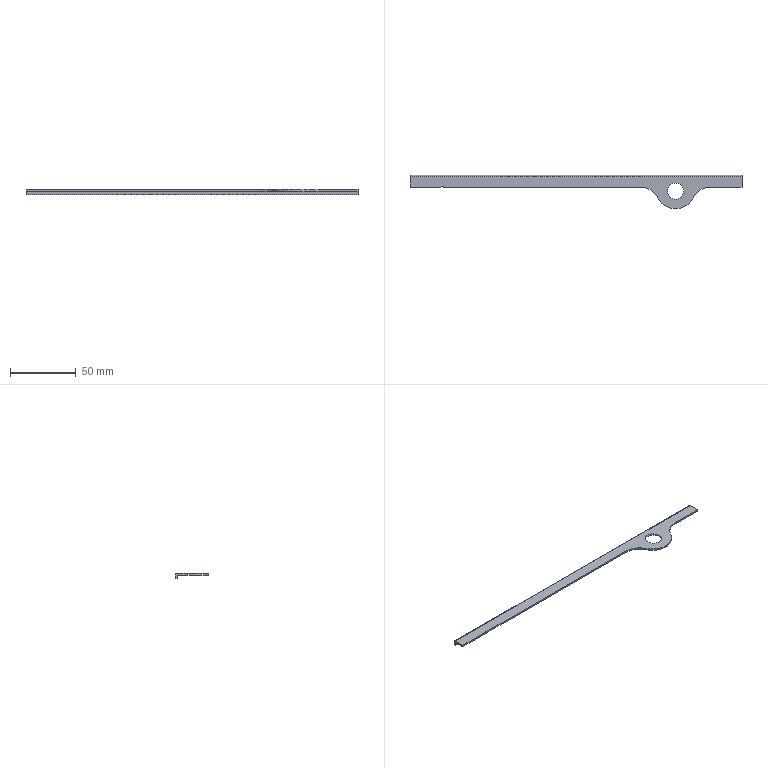Part | STEP file | gslz 2016.10.28-13_id1034_x_t | 1 solid | 17 faces | box 253.449 x 25.5 x 4 mm | volume 4072 mm3 | plane 10 | cylinder 7 | commonest cylinder face diameters 30 x3 4 x2 2 x1 12.3 x1
STEP:
#1=CARTESIAN_POINT('',(0.,0.,0.));
#2=DIRECTION('',(0.,0.,1.));
#3=DIRECTION('',(1.,0.,0.));
#4=AXIS2_PLACEMENT_3D('',#1,#2,#3);
#5=CARTESIAN_POINT('',(1262.778,254.,1.25));
#6=VERTEX_POINT('',#5);
#7=CARTESIAN_POINT('',(1256.628,254.,1.25));
#8=DIRECTION('',(0.,0.,1.));
#9=DIRECTION('',(1.,0.,0.));
#10=AXIS2_PLACEMENT_3D('',#7,#8,#9);
#11=CIRCLE('',#10,6.15);
#12=CARTESIAN_POINT('',(1256.628,254.,2.5));
#13=DIRECTION('',(0.,0.,-1.));
#14=DIRECTION('',(-1.,0.,0.));
#15=AXIS2_PLACEMENT_3D('',#12,#13,#14);
#16=CYLINDRICAL_SURFACE('',#15,6.15);
#17=CARTESIAN_POINT('',(9.425,1.25));
#18=DIRECTION('',(-1.,0.));
#19=VECTOR('',#18,1.);
#20=LINE('',#17,#19);
#21=(GEOMETRIC_REPRESENTATION_CONTEXT(2)PARAMETRIC_REPRESENTATION_CONTEXT()REPRESENTATION_CONTEXT('',''));
#22=DEFINITIONAL_REPRESENTATION('',(#20),#21);
#23=PCURVE('',#16,#22);
#24=CARTESIAN_POINT('',(3468.591,331.067,1.25));
#25=DIRECTION('',(0.,0.,1.));
#26=DIRECTION('',(1.,0.,0.));
#27=AXIS2_PLACEMENT_3D('',#24,#25,#26);
#28=PLANE('',#27);
#29=CARTESIAN_POINT('',(-2211.964,-77.067));
#30=DIRECTION('',(1.,0.));
#31=AXIS2_PLACEMENT_2D('',#29,#30);
#32=CIRCLE('',#31,6.15);
#33=(GEOMETRIC_REPRESENTATION_CONTEXT(2)PARAMETRIC_REPRESENTATION_CONTEXT()REPRESENTATION_CONTEXT('',''));
#34=DEFINITIONAL_REPRESENTATION('',(#32),#33);
#35=PCURVE('',#28,#34);
#36=SURFACE_CURVE('',#11,(#23,#35),.PCURVE_S1.);
#37=EDGE_CURVE('',#6,#6,#36,.T.);
#38=ORIENTED_EDGE('',*,*,#37,.F.);
#39=CARTESIAN_POINT('',(1262.778,254.,0.));
#40=VERTEX_POINT('',#39);
#41=CARTESIAN_POINT('',(1262.778,254.,1.25));
#42=CARTESIAN_POINT('',(1262.778,254.,0.));
#43=B_SPLINE_CURVE_WITH_KNOTS('',1,(#41,#42),.UNSPECIFIED.,.F.,.F.,(2,2),(1.25,2.5),.PIECEWISE_BEZIER_KNOTS.);
#44=CARTESIAN_POINT('',(9.425,0.));
#45=DIRECTION('',(0.,1.));
#46=VECTOR('',#45,1.);
#47=LINE('',#44,#46);
#48=(GEOMETRIC_REPRESENTATION_CONTEXT(2)PARAMETRIC_REPRESENTATION_CONTEXT()REPRESENTATION_CONTEXT('',''));
#49=DEFINITIONAL_REPRESENTATION('',(#47),#48);
#50=PCURVE('',#16,#49);
#51=CARTESIAN_POINT('',(3.142,0.));
#52=DIRECTION('',(0.,1.));
#53=VECTOR('',#52,1.);
#54=LINE('',#51,#53);
#55=(GEOMETRIC_REPRESENTATION_CONTEXT(2)PARAMETRIC_REPRESENTATION_CONTEXT()REPRESENTATION_CONTEXT('',''));
#56=DEFINITIONAL_REPRESENTATION('',(#54),#55);
#57=PCURVE('',#16,#56);
#58=SEAM_CURVE('',#43,(#50,#57),.PCURVE_S1.);
#59=EDGE_CURVE('',#6,#40,#58,.T.);
#60=ORIENTED_EDGE('',*,*,#59,.T.);
#61=CARTESIAN_POINT('',(1256.628,254.,0.));
#62=DIRECTION('',(0.,0.,-1.));
#63=DIRECTION('',(1.,0.,0.));
#64=AXIS2_PLACEMENT_3D('',#61,#62,#63);
#65=CIRCLE('',#64,6.15);
#66=CARTESIAN_POINT('',(3.142,2.5));
#67=DIRECTION('',(1.,0.));
#68=VECTOR('',#67,1.);
#69=LINE('',#66,#68);
#70=(GEOMETRIC_REPRESENTATION_CONTEXT(2)PARAMETRIC_REPRESENTATION_CONTEXT()REPRESENTATION_CONTEXT('',''));
#71=DEFINITIONAL_REPRESENTATION('',(#69),#70);
#72=PCURVE('',#16,#71);
#73=CARTESIAN_POINT('',(3468.591,331.067,0.));
#74=DIRECTION('',(0.,0.,1.));
#75=DIRECTION('',(1.,0.,0.));
#76=AXIS2_PLACEMENT_3D('',#73,#74,#75);
#77=PLANE('',#76);
#78=CARTESIAN_POINT('',(-2205.814,-77.067));
#79=CARTESIAN_POINT('',(-2205.814,-87.719));
#80=CARTESIAN_POINT('',(-2215.039,-82.393));
#81=CARTESIAN_POINT('',(-2224.264,-77.067));
#82=CARTESIAN_POINT('',(-2215.039,-71.741));
#83=CARTESIAN_POINT('',(-2205.814,-66.415));
#84=CARTESIAN_POINT('',(-2205.814,-77.067));
#85=(BOUNDED_CURVE()B_SPLINE_CURVE(2,(#78,#79,#80,#81,#82,#83,#84),.UNSPECIFIED.,.T.,.F.)B_SPLINE_CURVE_WITH_KNOTS((1,2,2,2,2,1),(-2.094,0.,2.094,4.189,6.283,8.378),.UNSPECIFIED.)CURVE()GEOMETRIC_REPRESENTATION_ITEM()RATIONAL_B_SPLINE_CURVE((1.,0.5,1.,0.5,1.,0.5,1.))REPRESENTATION_ITEM(''));
#86=(GEOMETRIC_REPRESENTATION_CONTEXT(2)PARAMETRIC_REPRESENTATION_CONTEXT()REPRESENTATION_CONTEXT('',''));
#87=DEFINITIONAL_REPRESENTATION('',(#85),#86);
#88=PCURVE('',#77,#87);
#89=SURFACE_CURVE('',#65,(#72,#88),.PCURVE_S1.);
#90=EDGE_CURVE('',#40,#40,#89,.T.);
#91=ORIENTED_EDGE('',*,*,#90,.F.);
#92=ORIENTED_EDGE('',*,*,#59,.F.);
#93=EDGE_LOOP('',(#38,#60,#91,#92));
#94=FACE_BOUND('',#93,.F.);
#95=ADVANCED_FACE('',(#94),#16,.F.);
#96=CARTESIAN_POINT('',(1077.412,257.,1.25));
#97=VERTEX_POINT('',#96);
#98=CARTESIAN_POINT('',(1053.925,257.,1.25));
#99=VERTEX_POINT('',#98);
#100=CARTESIAN_POINT('',(3468.591,257.,1.25));
#101=DIRECTION('',(-1.,0.,0.));
#102=VECTOR('',#101,1.);
#103=LINE('',#100,#102);
#104=CARTESIAN_POINT('',(1000.415,257.,2.5));
#105=DIRECTION('',(0.,1.,0.));
#106=DIRECTION('',(0.,0.,1.));
#107=AXIS2_PLACEMENT_3D('',#104,#105,#106);
#108=PLANE('',#107);
#109=CARTESIAN_POINT('',(-1.25,2468.176));
#110=DIRECTION('',(0.,-1.));
#111=VECTOR('',#110,1.);
#112=LINE('',#109,#111);
#113=(GEOMETRIC_REPRESENTATION_CONTEXT(2)PARAMETRIC_REPRESENTATION_CONTEXT()REPRESENTATION_CONTEXT('',''));
#114=DEFINITIONAL_REPRESENTATION('',(#112),#113);
#115=PCURVE('',#108,#114);
#116=CARTESIAN_POINT('',(0.,-74.067));
#117=DIRECTION('',(-1.,0.));
#118=VECTOR('',#117,1.);
#119=LINE('',#116,#118);
#120=(GEOMETRIC_REPRESENTATION_CONTEXT(2)PARAMETRIC_REPRESENTATION_CONTEXT()REPRESENTATION_CONTEXT('',''));
#121=DEFINITIONAL_REPRESENTATION('',(#119),#120);
#122=PCURVE('',#28,#121);
#123=SURFACE_CURVE('',#103,(#115,#122),.PCURVE_S1.);
#124=EDGE_CURVE('',#97,#99,#123,.T.);
#125=ORIENTED_EDGE('',*,*,#124,.T.);
#126=CARTESIAN_POINT('',(1053.925,257.,0.));
#127=VERTEX_POINT('',#126);
#128=CARTESIAN_POINT('',(1053.925,257.,2.5));
#129=DIRECTION('',(0.,0.,1.));
#130=VECTOR('',#129,1.);
#131=LINE('',#128,#130);
#132=CARTESIAN_POINT('',(0.,53.51));
#133=DIRECTION('',(1.,0.));
#134=VECTOR('',#133,1.);
#135=LINE('',#132,#134);
#136=(GEOMETRIC_REPRESENTATION_CONTEXT(2)PARAMETRIC_REPRESENTATION_CONTEXT()REPRESENTATION_CONTEXT('',''));
#137=DEFINITIONAL_REPRESENTATION('',(#135),#136);
#138=PCURVE('',#108,#137);
#139=CARTESIAN_POINT('',(1053.925,261.5,-0.75));
#140=DIRECTION('',(1.,0.,0.));
#141=DIRECTION('',(0.,0.,-1.));
#142=AXIS2_PLACEMENT_3D('',#139,#140,#141);
#143=PLANE('',#142);
#144=CARTESIAN_POINT('',(-3.25,-4.5));
#145=DIRECTION('',(-1.,0.));
#146=VECTOR('',#145,1.);
#147=LINE('',#144,#146);
#148=(GEOMETRIC_REPRESENTATION_CONTEXT(2)PARAMETRIC_REPRESENTATION_CONTEXT()REPRESENTATION_CONTEXT('',''));
#149=DEFINITIONAL_REPRESENTATION('',(#147),#148);
#150=PCURVE('',#143,#149);
#151=SURFACE_CURVE('',#131,(#138,#150),.PCURVE_S1.);
#152=EDGE_CURVE('',#127,#99,#151,.T.);
#153=ORIENTED_EDGE('',*,*,#152,.F.);
#154=CARTESIAN_POINT('',(1077.412,257.,0.));
#155=VERTEX_POINT('',#154);
#156=CARTESIAN_POINT('',(989.415,257.,0.));
#157=DIRECTION('',(-1.,0.,0.));
#158=VECTOR('',#157,1.);
#159=LINE('',#156,#158);
#160=CARTESIAN_POINT('',(-2.5,-11.));
#161=DIRECTION('',(0.,-1.));
#162=VECTOR('',#161,1.);
#163=LINE('',#160,#162);
#164=(GEOMETRIC_REPRESENTATION_CONTEXT(2)PARAMETRIC_REPRESENTATION_CONTEXT()REPRESENTATION_CONTEXT('',''));
#165=DEFINITIONAL_REPRESENTATION('',(#163),#164);
#166=PCURVE('',#108,#165);
#167=CARTESIAN_POINT('',(-2479.176,-74.067));
#168=DIRECTION('',(-1.,0.));
#169=VECTOR('',#168,1.);
#170=LINE('',#167,#169);
#171=(GEOMETRIC_REPRESENTATION_CONTEXT(2)PARAMETRIC_REPRESENTATION_CONTEXT()REPRESENTATION_CONTEXT('',''));
#172=DEFINITIONAL_REPRESENTATION('',(#170),#171);
#173=PCURVE('',#77,#172);
#174=SURFACE_CURVE('',#159,(#166,#173),.PCURVE_S1.);
#175=EDGE_CURVE('',#155,#127,#174,.T.);
#176=ORIENTED_EDGE('',*,*,#175,.F.);
#177=CARTESIAN_POINT('',(1077.412,257.,2.5));
#178=DIRECTION('',(0.,0.,-1.));
#179=VECTOR('',#178,1.);
#180=LINE('',#177,#179);
#181=CARTESIAN_POINT('',(0.,76.997));
#182=DIRECTION('',(-1.,0.));
#183=VECTOR('',#182,1.);
#184=LINE('',#181,#183);
#185=(GEOMETRIC_REPRESENTATION_CONTEXT(2)PARAMETRIC_REPRESENTATION_CONTEXT()REPRESENTATION_CONTEXT('',''));
#186=DEFINITIONAL_REPRESENTATION('',(#184),#185);
#187=PCURVE('',#108,#186);
#188=CARTESIAN_POINT('',(1078.466,255.3,2.5));
#189=DIRECTION('',(0.,0.,-1.));
#190=DIRECTION('',(-1.,0.,0.));
#191=AXIS2_PLACEMENT_3D('',#188,#189,#190);
#192=CYLINDRICAL_SURFACE('',#191,2.);
#193=CARTESIAN_POINT('',(1.016,0.));
#194=DIRECTION('',(0.,1.));
#195=VECTOR('',#194,1.);
#196=LINE('',#193,#195);
#197=(GEOMETRIC_REPRESENTATION_CONTEXT(2)PARAMETRIC_REPRESENTATION_CONTEXT()REPRESENTATION_CONTEXT('',''));
#198=DEFINITIONAL_REPRESENTATION('',(#196),#197);
#199=PCURVE('',#192,#198);
#200=SURFACE_CURVE('',#180,(#187,#199),.PCURVE_S1.);
#201=EDGE_CURVE('',#97,#155,#200,.T.);
#202=ORIENTED_EDGE('',*,*,#201,.F.);
#203=EDGE_LOOP('',(#125,#153,#176,#202));
#204=FACE_BOUND('',#203,.T.);
#205=ADVANCED_FACE('',(#204),#108,.F.);
#206=CARTESIAN_POINT('',(1079.226,257.15,0.));
#207=VERTEX_POINT('',#206);
#208=CARTESIAN_POINT('',(1079.226,257.15,1.25));
#209=VERTEX_POINT('',#208);
#210=CARTESIAN_POINT('',(1079.226,257.15,2.5));
#211=DIRECTION('',(0.,0.,1.));
#212=VECTOR('',#211,1.);
#213=LINE('',#210,#212);
#214=CARTESIAN_POINT('',(1.961,0.));
#215=DIRECTION('',(0.,-1.));
#216=VECTOR('',#215,1.);
#217=LINE('',#214,#216);
#218=(GEOMETRIC_REPRESENTATION_CONTEXT(2)PARAMETRIC_REPRESENTATION_CONTEXT()REPRESENTATION_CONTEXT('',''));
#219=DEFINITIONAL_REPRESENTATION('',(#217),#218);
#220=PCURVE('',#192,#219);
#221=CARTESIAN_POINT('',(1079.985,259.,2.5));
#222=DIRECTION('',(0.,0.,-1.));
#223=DIRECTION('',(-1.,0.,0.));
#224=AXIS2_PLACEMENT_3D('',#221,#222,#223);
#225=CYLINDRICAL_SURFACE('',#224,2.);
#226=CARTESIAN_POINT('',(5.102,0.));
#227=DIRECTION('',(0.,-1.));
#228=VECTOR('',#227,1.);
#229=LINE('',#226,#228);
#230=(GEOMETRIC_REPRESENTATION_CONTEXT(2)PARAMETRIC_REPRESENTATION_CONTEXT()REPRESENTATION_CONTEXT('',''));
#231=DEFINITIONAL_REPRESENTATION('',(#229),#230);
#232=PCURVE('',#225,#231);
#233=SURFACE_CURVE('',#213,(#220,#232),.PCURVE_S1.);
#234=EDGE_CURVE('',#207,#209,#233,.T.);
#235=ORIENTED_EDGE('',*,*,#234,.F.);
#236=CARTESIAN_POINT('',(1078.466,255.3,0.));
#237=DIRECTION('',(0.,0.,-1.));
#238=DIRECTION('',(1.,0.,0.));
#239=AXIS2_PLACEMENT_3D('',#236,#237,#238);
#240=CIRCLE('',#239,2.);
#241=CARTESIAN_POINT('',(-3.142,2.5));
#242=DIRECTION('',(1.,0.));
#243=VECTOR('',#242,1.);
#244=LINE('',#241,#243);
#245=(GEOMETRIC_REPRESENTATION_CONTEXT(2)PARAMETRIC_REPRESENTATION_CONTEXT()REPRESENTATION_CONTEXT('',''));
#246=DEFINITIONAL_REPRESENTATION('',(#244),#245);
#247=PCURVE('',#192,#246);
#248=CARTESIAN_POINT('',(-2388.126,-75.767));
#249=CARTESIAN_POINT('',(-2388.126,-79.231));
#250=CARTESIAN_POINT('',(-2391.126,-77.499));
#251=CARTESIAN_POINT('',(-2394.126,-75.767));
#252=CARTESIAN_POINT('',(-2391.126,-74.035));
#253=CARTESIAN_POINT('',(-2388.126,-72.303));
#254=CARTESIAN_POINT('',(-2388.126,-75.767));
#255=(BOUNDED_CURVE()B_SPLINE_CURVE(2,(#248,#249,#250,#251,#252,#253,#254),.UNSPECIFIED.,.T.,.F.)B_SPLINE_CURVE_WITH_KNOTS((1,2,2,2,2,1),(-2.094,0.,2.094,4.189,6.283,8.378),.UNSPECIFIED.)CURVE()GEOMETRIC_REPRESENTATION_ITEM()RATIONAL_B_SPLINE_CURVE((1.,0.5,1.,0.5,1.,0.5,1.))REPRESENTATION_ITEM(''));
#256=(GEOMETRIC_REPRESENTATION_CONTEXT(2)PARAMETRIC_REPRESENTATION_CONTEXT()REPRESENTATION_CONTEXT('',''));
#257=DEFINITIONAL_REPRESENTATION('',(#255),#256);
#258=PCURVE('',#77,#257);
#259=SURFACE_CURVE('',#240,(#247,#258),.PCURVE_S1.);
#260=EDGE_CURVE('',#155,#207,#259,.T.);
#261=ORIENTED_EDGE('',*,*,#260,.F.);
#262=ORIENTED_EDGE('',*,*,#201,.F.);
#263=CARTESIAN_POINT('',(1078.466,255.3,1.25));
#264=DIRECTION('',(0.,0.,1.));
#265=DIRECTION('',(1.,0.,0.));
#266=AXIS2_PLACEMENT_3D('',#263,#264,#265);
#267=CIRCLE('',#266,2.);
#268=CARTESIAN_POINT('',(3.142,1.25));
#269=DIRECTION('',(-1.,0.));
#270=VECTOR('',#269,1.);
#271=LINE('',#268,#270);
#272=(GEOMETRIC_REPRESENTATION_CONTEXT(2)PARAMETRIC_REPRESENTATION_CONTEXT()REPRESENTATION_CONTEXT('',''));
#273=DEFINITIONAL_REPRESENTATION('',(#271),#272);
#274=PCURVE('',#192,#273);
#275=CARTESIAN_POINT('',(-2390.126,-75.767));
#276=DIRECTION('',(1.,0.));
#277=AXIS2_PLACEMENT_2D('',#275,#276);
#278=CIRCLE('',#277,2.);
#279=(GEOMETRIC_REPRESENTATION_CONTEXT(2)PARAMETRIC_REPRESENTATION_CONTEXT()REPRESENTATION_CONTEXT('',''));
#280=DEFINITIONAL_REPRESENTATION('',(#278),#279);
#281=PCURVE('',#28,#280);
#282=SURFACE_CURVE('',#267,(#274,#281),.PCURVE_S1.);
#283=EDGE_CURVE('',#209,#97,#282,.T.);
#284=ORIENTED_EDGE('',*,*,#283,.F.);
#285=EDGE_LOOP('',(#235,#261,#262,#284));
#286=FACE_BOUND('',#285,.F.);
#287=ADVANCED_FACE('',(#286),#192,.F.);
#288=CARTESIAN_POINT('',(1079.985,257.,1.25));
#289=VERTEX_POINT('',#288);
#290=CARTESIAN_POINT('',(1079.985,259.,1.25));
#291=DIRECTION('',(0.,0.,-1.));
#292=DIRECTION('',(1.,0.,0.));
#293=AXIS2_PLACEMENT_3D('',#290,#291,#292);
#294=CIRCLE('',#293,2.);
#295=CARTESIAN_POINT('',(3.142,1.25));
#296=DIRECTION('',(1.,0.));
#297=VECTOR('',#296,1.);
#298=LINE('',#295,#297);
#299=(GEOMETRIC_REPRESENTATION_CONTEXT(2)PARAMETRIC_REPRESENTATION_CONTEXT()REPRESENTATION_CONTEXT('',''));
#300=DEFINITIONAL_REPRESENTATION('',(#298),#299);
#301=PCURVE('',#225,#300);
#302=CARTESIAN_POINT('',(-2386.606,-72.067));
#303=CARTESIAN_POINT('',(-2386.606,-75.531));
#304=CARTESIAN_POINT('',(-2389.606,-73.799));
#305=CARTESIAN_POINT('',(-2392.606,-72.067));
#306=CARTESIAN_POINT('',(-2389.606,-70.335));
#307=CARTESIAN_POINT('',(-2386.606,-68.603));
#308=CARTESIAN_POINT('',(-2386.606,-72.067));
#309=(BOUNDED_CURVE()B_SPLINE_CURVE(2,(#302,#303,#304,#305,#306,#307,#308),.UNSPECIFIED.,.T.,.F.)B_SPLINE_CURVE_WITH_KNOTS((1,2,2,2,2,1),(-2.094,0.,2.094,4.189,6.283,8.378),.UNSPECIFIED.)CURVE()GEOMETRIC_REPRESENTATION_ITEM()RATIONAL_B_SPLINE_CURVE((1.,0.5,1.,0.5,1.,0.5,1.))REPRESENTATION_ITEM(''));
#310=(GEOMETRIC_REPRESENTATION_CONTEXT(2)PARAMETRIC_REPRESENTATION_CONTEXT()REPRESENTATION_CONTEXT('',''));
#311=DEFINITIONAL_REPRESENTATION('',(#309),#310);
#312=PCURVE('',#28,#311);
#313=SURFACE_CURVE('',#294,(#301,#312),.PCURVE_S1.);
#314=EDGE_CURVE('',#289,#209,#313,.T.);
#315=ORIENTED_EDGE('',*,*,#314,.T.);
#316=ORIENTED_EDGE('',*,*,#234,.F.);
#317=CARTESIAN_POINT('',(1079.985,257.,0.));
#318=VERTEX_POINT('',#317);
#319=CARTESIAN_POINT('',(1079.985,259.,0.));
#320=DIRECTION('',(0.,0.,1.));
#321=DIRECTION('',(1.,0.,0.));
#322=AXIS2_PLACEMENT_3D('',#319,#320,#321);
#323=CIRCLE('',#322,2.);
#324=CARTESIAN_POINT('',(9.425,2.5));
#325=DIRECTION('',(-1.,0.));
#326=VECTOR('',#325,1.);
#327=LINE('',#324,#326);
#328=(GEOMETRIC_REPRESENTATION_CONTEXT(2)PARAMETRIC_REPRESENTATION_CONTEXT()REPRESENTATION_CONTEXT('',''));
#329=DEFINITIONAL_REPRESENTATION('',(#327),#328);
#330=PCURVE('',#225,#329);
#331=CARTESIAN_POINT('',(-2388.606,-72.067));
#332=DIRECTION('',(1.,0.));
#333=AXIS2_PLACEMENT_2D('',#331,#332);
#334=CIRCLE('',#333,2.);
#335=(GEOMETRIC_REPRESENTATION_CONTEXT(2)PARAMETRIC_REPRESENTATION_CONTEXT()REPRESENTATION_CONTEXT('',''));
#336=DEFINITIONAL_REPRESENTATION('',(#334),#335);
#337=PCURVE('',#77,#336);
#338=SURFACE_CURVE('',#323,(#330,#337),.PCURVE_S1.);
#339=EDGE_CURVE('',#207,#318,#338,.T.);
#340=ORIENTED_EDGE('',*,*,#339,.T.);
#341=CARTESIAN_POINT('',(1079.985,257.,2.5));
#342=DIRECTION('',(0.,0.,1.));
#343=VECTOR('',#342,1.);
#344=LINE('',#341,#343);
#345=CARTESIAN_POINT('',(4.712,0.));
#346=DIRECTION('',(0.,-1.));
#347=VECTOR('',#346,1.);
#348=LINE('',#345,#347);
#349=(GEOMETRIC_REPRESENTATION_CONTEXT(2)PARAMETRIC_REPRESENTATION_CONTEXT()REPRESENTATION_CONTEXT('',''));
#350=DEFINITIONAL_REPRESENTATION('',(#348),#349);
#351=PCURVE('',#225,#350);
#352=CARTESIAN_POINT('',(1228.343,257.,2.5));
#353=DIRECTION('',(0.,-1.,0.));
#354=DIRECTION('',(1.,0.,0.));
#355=AXIS2_PLACEMENT_3D('',#352,#353,#354);
#356=PLANE('',#355);
#357=CARTESIAN_POINT('',(-148.358,0.));
#358=DIRECTION('',(0.,1.));
#359=VECTOR('',#358,1.);
#360=LINE('',#357,#359);
#361=(GEOMETRIC_REPRESENTATION_CONTEXT(2)PARAMETRIC_REPRESENTATION_CONTEXT()REPRESENTATION_CONTEXT('',''));
#362=DEFINITIONAL_REPRESENTATION('',(#360),#361);
#363=PCURVE('',#356,#362);
#364=SURFACE_CURVE('',#344,(#351,#363),.PCURVE_S1.);
#365=EDGE_CURVE('',#318,#289,#364,.T.);
#366=ORIENTED_EDGE('',*,*,#365,.T.);
#367=EDGE_LOOP('',(#315,#316,#340,#366));
#368=FACE_BOUND('',#367,.T.);
#369=ADVANCED_FACE('',(#368),#225,.T.);
#370=CARTESIAN_POINT('',(1229.837,257.,0.));
#371=VERTEX_POINT('',#370);
#372=CARTESIAN_POINT('',(1228.343,257.,0.));
#373=DIRECTION('',(-1.,0.,0.));
#374=VECTOR('',#373,1.);
#375=LINE('',#372,#374);
#376=CARTESIAN_POINT('',(0.,-2.5));
#377=DIRECTION('',(-1.,0.));
#378=VECTOR('',#377,1.);
#379=LINE('',#376,#378);
#380=(GEOMETRIC_REPRESENTATION_CONTEXT(2)PARAMETRIC_REPRESENTATION_CONTEXT()REPRESENTATION_CONTEXT('',''));
#381=DEFINITIONAL_REPRESENTATION('',(#379),#380);
#382=PCURVE('',#356,#381);
#383=CARTESIAN_POINT('',(-2240.248,-74.067));
#384=DIRECTION('',(-1.,0.));
#385=VECTOR('',#384,1.);
#386=LINE('',#383,#385);
#387=(GEOMETRIC_REPRESENTATION_CONTEXT(2)PARAMETRIC_REPRESENTATION_CONTEXT()REPRESENTATION_CONTEXT('',''));
#388=DEFINITIONAL_REPRESENTATION('',(#386),#387);
#389=PCURVE('',#77,#388);
#390=SURFACE_CURVE('',#375,(#382,#389),.PCURVE_S1.);
#391=EDGE_CURVE('',#371,#318,#390,.T.);
#392=ORIENTED_EDGE('',*,*,#391,.F.);
#393=CARTESIAN_POINT('',(1229.837,257.,1.25));
#394=VERTEX_POINT('',#393);
#395=CARTESIAN_POINT('',(1229.837,257.,2.5));
#396=DIRECTION('',(0.,0.,1.));
#397=VECTOR('',#396,1.);
#398=LINE('',#395,#397);
#399=CARTESIAN_POINT('',(1.493,0.));
#400=DIRECTION('',(0.,1.));
#401=VECTOR('',#400,1.);
#402=LINE('',#399,#401);
#403=(GEOMETRIC_REPRESENTATION_CONTEXT(2)PARAMETRIC_REPRESENTATION_CONTEXT()REPRESENTATION_CONTEXT('',''));
#404=DEFINITIONAL_REPRESENTATION('',(#402),#403);
#405=PCURVE('',#356,#404);
#406=CARTESIAN_POINT('',(1229.837,242.,2.5));
#407=DIRECTION('',(0.,0.,-1.));
#408=DIRECTION('',(-1.,0.,0.));
#409=AXIS2_PLACEMENT_3D('',#406,#407,#408);
#410=CYLINDRICAL_SURFACE('',#409,15.);
#411=CARTESIAN_POINT('',(1.571,0.));
#412=DIRECTION('',(0.,-1.));
#413=VECTOR('',#412,1.);
#414=LINE('',#411,#413);
#415=(GEOMETRIC_REPRESENTATION_CONTEXT(2)PARAMETRIC_REPRESENTATION_CONTEXT()REPRESENTATION_CONTEXT('',''));
#416=DEFINITIONAL_REPRESENTATION('',(#414),#415);
#417=PCURVE('',#410,#416);
#418=SURFACE_CURVE('',#398,(#405,#417),.PCURVE_S1.);
#419=EDGE_CURVE('',#371,#394,#418,.T.);
#420=ORIENTED_EDGE('',*,*,#419,.T.);
#421=CARTESIAN_POINT('',(3468.591,257.,1.25));
#422=DIRECTION('',(-1.,0.,0.));
#423=VECTOR('',#422,1.);
#424=LINE('',#421,#423);
#425=CARTESIAN_POINT('',(2240.248,-1.25));
#426=DIRECTION('',(-1.,0.));
#427=VECTOR('',#426,1.);
#428=LINE('',#425,#427);
#429=(GEOMETRIC_REPRESENTATION_CONTEXT(2)PARAMETRIC_REPRESENTATION_CONTEXT()REPRESENTATION_CONTEXT('',''));
#430=DEFINITIONAL_REPRESENTATION('',(#428),#429);
#431=PCURVE('',#356,#430);
#432=CARTESIAN_POINT('',(0.,-74.067));
#433=DIRECTION('',(-1.,0.));
#434=VECTOR('',#433,1.);
#435=LINE('',#432,#434);
#436=(GEOMETRIC_REPRESENTATION_CONTEXT(2)PARAMETRIC_REPRESENTATION_CONTEXT()REPRESENTATION_CONTEXT('',''));
#437=DEFINITIONAL_REPRESENTATION('',(#435),#436);
#438=PCURVE('',#28,#437);
#439=SURFACE_CURVE('',#424,(#431,#438),.PCURVE_S1.);
#440=EDGE_CURVE('',#394,#289,#439,.T.);
#441=ORIENTED_EDGE('',*,*,#440,.T.);
#442=ORIENTED_EDGE('',*,*,#365,.F.);
#443=EDGE_LOOP('',(#392,#420,#441,#442));
#444=FACE_BOUND('',#443,.T.);
#445=ADVANCED_FACE('',(#444),#356,.T.);
#446=CARTESIAN_POINT('',(1243.232,248.75,1.25));
#447=VERTEX_POINT('',#446);
#448=CARTESIAN_POINT('',(1229.837,242.,1.25));
#449=DIRECTION('',(0.,0.,-1.));
#450=DIRECTION('',(1.,0.,0.));
#451=AXIS2_PLACEMENT_3D('',#448,#449,#450);
#452=CIRCLE('',#451,15.);
#453=CARTESIAN_POINT('',(-3.142,1.25));
#454=DIRECTION('',(1.,0.));
#455=VECTOR('',#454,1.);
#456=LINE('',#453,#455);
#457=(GEOMETRIC_REPRESENTATION_CONTEXT(2)PARAMETRIC_REPRESENTATION_CONTEXT()REPRESENTATION_CONTEXT('',''));
#458=DEFINITIONAL_REPRESENTATION('',(#456),#457);
#459=PCURVE('',#410,#458);
#460=CARTESIAN_POINT('',(-2223.754,-89.067));
#461=CARTESIAN_POINT('',(-2223.754,-115.047));
#462=CARTESIAN_POINT('',(-2246.254,-102.057));
#463=CARTESIAN_POINT('',(-2268.754,-89.067));
#464=CARTESIAN_POINT('',(-2246.254,-76.076));
#465=CARTESIAN_POINT('',(-2223.754,-63.086));
#466=CARTESIAN_POINT('',(-2223.754,-89.067));
#467=(BOUNDED_CURVE()B_SPLINE_CURVE(2,(#460,#461,#462,#463,#464,#465,#466),.UNSPECIFIED.,.T.,.F.)B_SPLINE_CURVE_WITH_KNOTS((1,2,2,2,2,1),(-2.094,0.,2.094,4.189,6.283,8.378),.UNSPECIFIED.)CURVE()GEOMETRIC_REPRESENTATION_ITEM()RATIONAL_B_SPLINE_CURVE((1.,0.5,1.,0.5,1.,0.5,1.))REPRESENTATION_ITEM(''));
#468=(GEOMETRIC_REPRESENTATION_CONTEXT(2)PARAMETRIC_REPRESENTATION_CONTEXT()REPRESENTATION_CONTEXT('',''));
#469=DEFINITIONAL_REPRESENTATION('',(#467),#468);
#470=PCURVE('',#28,#469);
#471=SURFACE_CURVE('',#452,(#459,#470),.PCURVE_S1.);
#472=EDGE_CURVE('',#394,#447,#471,.T.);
#473=ORIENTED_EDGE('',*,*,#472,.T.);
#474=CARTESIAN_POINT('',(1243.232,248.75,0.));
#475=VERTEX_POINT('',#474);
#476=CARTESIAN_POINT('',(1243.232,248.75,0.625));
#477=DIRECTION('',(0.,0.,1.));
#478=VECTOR('',#477,1.);
#479=LINE('',#476,#478);
#480=CARTESIAN_POINT('',(2.675,1.875));
#481=DIRECTION('',(0.,-1.));
#482=VECTOR('',#481,1.);
#483=LINE('',#480,#482);
#484=(GEOMETRIC_REPRESENTATION_CONTEXT(2)PARAMETRIC_REPRESENTATION_CONTEXT()REPRESENTATION_CONTEXT('',''));
#485=DEFINITIONAL_REPRESENTATION('',(#483),#484);
#486=PCURVE('',#410,#485);
#487=CARTESIAN_POINT('',(1256.628,255.5,2.5));
#488=DIRECTION('',(0.,0.,-1.));
#489=DIRECTION('',(-1.,0.,0.));
#490=AXIS2_PLACEMENT_3D('',#487,#488,#489);
#491=CYLINDRICAL_SURFACE('',#490,15.);
#492=CARTESIAN_POINT('',(5.816,1.875));
#493=DIRECTION('',(0.,-1.));
#494=VECTOR('',#493,1.);
#495=LINE('',#492,#494);
#496=(GEOMETRIC_REPRESENTATION_CONTEXT(2)PARAMETRIC_REPRESENTATION_CONTEXT()REPRESENTATION_CONTEXT('',''));
#497=DEFINITIONAL_REPRESENTATION('',(#495),#496);
#498=PCURVE('',#491,#497);
#499=SURFACE_CURVE('',#479,(#486,#498),.PCURVE_S1.);
#500=EDGE_CURVE('',#475,#447,#499,.T.);
#501=ORIENTED_EDGE('',*,*,#500,.F.);
#502=CARTESIAN_POINT('',(1229.837,242.,0.));
#503=DIRECTION('',(0.,0.,1.));
#504=DIRECTION('',(1.,0.,0.));
#505=AXIS2_PLACEMENT_3D('',#502,#503,#504);
#506=CIRCLE('',#505,15.);
#507=CARTESIAN_POINT('',(3.142,2.5));
#508=DIRECTION('',(-1.,0.));
#509=VECTOR('',#508,1.);
#510=LINE('',#507,#509);
#511=(GEOMETRIC_REPRESENTATION_CONTEXT(2)PARAMETRIC_REPRESENTATION_CONTEXT()REPRESENTATION_CONTEXT('',''));
#512=DEFINITIONAL_REPRESENTATION('',(#510),#511);
#513=PCURVE('',#410,#512);
#514=CARTESIAN_POINT('',(-2238.754,-89.067));
#515=DIRECTION('',(1.,0.));
#516=AXIS2_PLACEMENT_2D('',#514,#515);
#517=CIRCLE('',#516,15.);
#518=(GEOMETRIC_REPRESENTATION_CONTEXT(2)PARAMETRIC_REPRESENTATION_CONTEXT()REPRESENTATION_CONTEXT('',''));
#519=DEFINITIONAL_REPRESENTATION('',(#517),#518);
#520=PCURVE('',#77,#519);
#521=SURFACE_CURVE('',#506,(#513,#520),.PCURVE_S1.);
#522=EDGE_CURVE('',#475,#371,#521,.T.);
#523=ORIENTED_EDGE('',*,*,#522,.T.);
#524=ORIENTED_EDGE('',*,*,#419,.T.);
#525=EDGE_LOOP('',(#473,#501,#523,#524));
#526=FACE_BOUND('',#525,.F.);
#527=ADVANCED_FACE('',(#526),#410,.F.);
#528=CARTESIAN_POINT('',(1270.023,248.75,0.));
#529=VERTEX_POINT('',#528);
#530=CARTESIAN_POINT('',(1256.628,255.5,0.));
#531=DIRECTION('',(0.,0.,-1.));
#532=DIRECTION('',(1.,0.,0.));
#533=AXIS2_PLACEMENT_3D('',#530,#531,#532);
#534=CIRCLE('',#533,15.);
#535=CARTESIAN_POINT('',(3.142,2.5));
#536=DIRECTION('',(1.,0.));
#537=VECTOR('',#536,1.);
#538=LINE('',#535,#537);
#539=(GEOMETRIC_REPRESENTATION_CONTEXT(2)PARAMETRIC_REPRESENTATION_CONTEXT()REPRESENTATION_CONTEXT('',''));
#540=DEFINITIONAL_REPRESENTATION('',(#538),#539);
#541=PCURVE('',#491,#540);
#542=CARTESIAN_POINT('',(-2196.964,-75.567));
#543=CARTESIAN_POINT('',(-2196.964,-101.547));
#544=CARTESIAN_POINT('',(-2219.464,-88.557));
#545=CARTESIAN_POINT('',(-2241.964,-75.567));
#546=CARTESIAN_POINT('',(-2219.464,-62.576));
#547=CARTESIAN_POINT('',(-2196.964,-49.586));
#548=CARTESIAN_POINT('',(-2196.964,-75.567));
#549=(BOUNDED_CURVE()B_SPLINE_CURVE(2,(#542,#543,#544,#545,#546,#547,#548),.UNSPECIFIED.,.T.,.F.)B_SPLINE_CURVE_WITH_KNOTS((1,2,2,2,2,1),(-2.094,0.,2.094,4.189,6.283,8.378),.UNSPECIFIED.)CURVE()GEOMETRIC_REPRESENTATION_ITEM()RATIONAL_B_SPLINE_CURVE((1.,0.5,1.,0.5,1.,0.5,1.))REPRESENTATION_ITEM(''));
#550=(GEOMETRIC_REPRESENTATION_CONTEXT(2)PARAMETRIC_REPRESENTATION_CONTEXT()REPRESENTATION_CONTEXT('',''));
#551=DEFINITIONAL_REPRESENTATION('',(#549),#550);
#552=PCURVE('',#77,#551);
#553=SURFACE_CURVE('',#534,(#541,#552),.PCURVE_S1.);
#554=EDGE_CURVE('',#529,#475,#553,.T.);
#555=ORIENTED_EDGE('',*,*,#554,.F.);
#556=CARTESIAN_POINT('',(1270.023,248.75,1.25));
#557=VERTEX_POINT('',#556);
#558=CARTESIAN_POINT('',(1270.023,248.75,0.625));
#559=DIRECTION('',(0.,0.,1.));
#560=VECTOR('',#559,1.);
#561=LINE('',#558,#560);
#562=CARTESIAN_POINT('',(3.608,1.875));
#563=DIRECTION('',(0.,-1.));
#564=VECTOR('',#563,1.);
#565=LINE('',#562,#564);
#566=(GEOMETRIC_REPRESENTATION_CONTEXT(2)PARAMETRIC_REPRESENTATION_CONTEXT()REPRESENTATION_CONTEXT('',''));
#567=DEFINITIONAL_REPRESENTATION('',(#565),#566);
#568=PCURVE('',#491,#567);
#569=CARTESIAN_POINT('',(1283.418,242.,2.5));
#570=DIRECTION('',(0.,0.,-1.));
#571=DIRECTION('',(-1.,0.,0.));
#572=AXIS2_PLACEMENT_3D('',#569,#570,#571);
#573=CYLINDRICAL_SURFACE('',#572,15.);
#574=CARTESIAN_POINT('',(0.4668,1.875));
#575=DIRECTION('',(0.,-1.));
#576=VECTOR('',#575,1.);
#577=LINE('',#574,#576);
#578=(GEOMETRIC_REPRESENTATION_CONTEXT(2)PARAMETRIC_REPRESENTATION_CONTEXT()REPRESENTATION_CONTEXT('',''));
#579=DEFINITIONAL_REPRESENTATION('',(#577),#578);
#580=PCURVE('',#573,#579);
#581=SURFACE_CURVE('',#561,(#568,#580),.PCURVE_S1.);
#582=EDGE_CURVE('',#529,#557,#581,.T.);
#583=ORIENTED_EDGE('',*,*,#582,.T.);
#584=CARTESIAN_POINT('',(1256.628,255.5,1.25));
#585=DIRECTION('',(0.,0.,1.));
#586=DIRECTION('',(1.,0.,0.));
#587=AXIS2_PLACEMENT_3D('',#584,#585,#586);
#588=CIRCLE('',#587,15.);
#589=CARTESIAN_POINT('',(9.425,1.25));
#590=DIRECTION('',(-1.,0.));
#591=VECTOR('',#590,1.);
#592=LINE('',#589,#591);
#593=(GEOMETRIC_REPRESENTATION_CONTEXT(2)PARAMETRIC_REPRESENTATION_CONTEXT()REPRESENTATION_CONTEXT('',''));
#594=DEFINITIONAL_REPRESENTATION('',(#592),#593);
#595=PCURVE('',#491,#594);
#596=CARTESIAN_POINT('',(-2211.964,-75.567));
#597=DIRECTION('',(1.,0.));
#598=AXIS2_PLACEMENT_2D('',#596,#597);
#599=CIRCLE('',#598,15.);
#600=(GEOMETRIC_REPRESENTATION_CONTEXT(2)PARAMETRIC_REPRESENTATION_CONTEXT()REPRESENTATION_CONTEXT('',''));
#601=DEFINITIONAL_REPRESENTATION('',(#599),#600);
#602=PCURVE('',#28,#601);
#603=SURFACE_CURVE('',#588,(#595,#602),.PCURVE_S1.);
#604=EDGE_CURVE('',#447,#557,#603,.T.);
#605=ORIENTED_EDGE('',*,*,#604,.F.);
#606=ORIENTED_EDGE('',*,*,#500,.F.);
#607=EDGE_LOOP('',(#555,#583,#605,#606));
#608=FACE_BOUND('',#607,.T.);
#609=ADVANCED_FACE('',(#608),#491,.T.);
#610=CARTESIAN_POINT('',(1283.418,257.,1.25));
#611=VERTEX_POINT('',#610);
#612=CARTESIAN_POINT('',(1283.418,242.,1.25));
#613=DIRECTION('',(0.,0.,-1.));
#614=DIRECTION('',(1.,0.,0.));
#615=AXIS2_PLACEMENT_3D('',#612,#613,#614);
#616=CIRCLE('',#615,15.);
#617=CARTESIAN_POINT('',(-3.142,1.25));
#618=DIRECTION('',(1.,0.));
#619=VECTOR('',#618,1.);
#620=LINE('',#617,#619);
#621=(GEOMETRIC_REPRESENTATION_CONTEXT(2)PARAMETRIC_REPRESENTATION_CONTEXT()REPRESENTATION_CONTEXT('',''));
#622=DEFINITIONAL_REPRESENTATION('',(#620),#621);
#623=PCURVE('',#573,#622);
#624=CARTESIAN_POINT('',(-2170.173,-89.067));
#625=CARTESIAN_POINT('',(-2170.173,-115.047));
#626=CARTESIAN_POINT('',(-2192.673,-102.057));
#627=CARTESIAN_POINT('',(-2215.173,-89.067));
#628=CARTESIAN_POINT('',(-2192.673,-76.076));
#629=CARTESIAN_POINT('',(-2170.173,-63.086));
#630=CARTESIAN_POINT('',(-2170.173,-89.067));
#631=(BOUNDED_CURVE()B_SPLINE_CURVE(2,(#624,#625,#626,#627,#628,#629,#630),.UNSPECIFIED.,.T.,.F.)B_SPLINE_CURVE_WITH_KNOTS((1,2,2,2,2,1),(-2.094,0.,2.094,4.189,6.283,8.378),.UNSPECIFIED.)CURVE()GEOMETRIC_REPRESENTATION_ITEM()RATIONAL_B_SPLINE_CURVE((1.,0.5,1.,0.5,1.,0.5,1.))REPRESENTATION_ITEM(''));
#632=(GEOMETRIC_REPRESENTATION_CONTEXT(2)PARAMETRIC_REPRESENTATION_CONTEXT()REPRESENTATION_CONTEXT('',''));
#633=DEFINITIONAL_REPRESENTATION('',(#631),#632);
#634=PCURVE('',#28,#633);
#635=SURFACE_CURVE('',#616,(#623,#634),.PCURVE_S1.);
#636=EDGE_CURVE('',#557,#611,#635,.T.);
#637=ORIENTED_EDGE('',*,*,#636,.T.);
#638=CARTESIAN_POINT('',(1283.418,257.,0.));
#639=VERTEX_POINT('',#638);
#640=CARTESIAN_POINT('',(1283.418,257.,2.5));
#641=DIRECTION('',(0.,0.,1.));
#642=VECTOR('',#641,1.);
#643=LINE('',#640,#642);
#644=CARTESIAN_POINT('',(1.571,0.));
#645=DIRECTION('',(0.,-1.));
#646=VECTOR('',#645,1.);
#647=LINE('',#644,#646);
#648=(GEOMETRIC_REPRESENTATION_CONTEXT(2)PARAMETRIC_REPRESENTATION_CONTEXT()REPRESENTATION_CONTEXT('',''));
#649=DEFINITIONAL_REPRESENTATION('',(#647),#648);
#650=PCURVE('',#573,#649);
#651=CARTESIAN_POINT('',(1263.783,257.,0.));
#652=DIRECTION('',(0.,-1.,0.));
#653=DIRECTION('',(0.,0.,-1.));
#654=AXIS2_PLACEMENT_3D('',#651,#652,#653);
#655=PLANE('',#654);
#656=CARTESIAN_POINT('',(-2.5,19.635));
#657=DIRECTION('',(-1.,0.));
#658=VECTOR('',#657,1.);
#659=LINE('',#656,#658);
#660=(GEOMETRIC_REPRESENTATION_CONTEXT(2)PARAMETRIC_REPRESENTATION_CONTEXT()REPRESENTATION_CONTEXT('',''));
#661=DEFINITIONAL_REPRESENTATION('',(#659),#660);
#662=PCURVE('',#655,#661);
#663=SURFACE_CURVE('',#643,(#650,#662),.PCURVE_S1.);
#664=EDGE_CURVE('',#639,#611,#663,.T.);
#665=ORIENTED_EDGE('',*,*,#664,.F.);
#666=CARTESIAN_POINT('',(1283.418,242.,0.));
#667=DIRECTION('',(0.,0.,1.));
#668=DIRECTION('',(1.,0.,0.));
#669=AXIS2_PLACEMENT_3D('',#666,#667,#668);
#670=CIRCLE('',#669,15.);
#671=CARTESIAN_POINT('',(3.142,2.5));
#672=DIRECTION('',(-1.,0.));
#673=VECTOR('',#672,1.);
#674=LINE('',#671,#673);
#675=(GEOMETRIC_REPRESENTATION_CONTEXT(2)PARAMETRIC_REPRESENTATION_CONTEXT()REPRESENTATION_CONTEXT('',''));
#676=DEFINITIONAL_REPRESENTATION('',(#674),#675);
#677=PCURVE('',#573,#676);
#678=CARTESIAN_POINT('',(-2185.173,-89.067));
#679=DIRECTION('',(1.,0.));
#680=AXIS2_PLACEMENT_2D('',#678,#679);
#681=CIRCLE('',#680,15.);
#682=(GEOMETRIC_REPRESENTATION_CONTEXT(2)PARAMETRIC_REPRESENTATION_CONTEXT()REPRESENTATION_CONTEXT('',''));
#683=DEFINITIONAL_REPRESENTATION('',(#681),#682);
#684=PCURVE('',#77,#683);
#685=SURFACE_CURVE('',#670,(#677,#684),.PCURVE_S1.);
#686=EDGE_CURVE('',#639,#529,#685,.T.);
#687=ORIENTED_EDGE('',*,*,#686,.T.);
#688=ORIENTED_EDGE('',*,*,#582,.T.);
#689=EDGE_LOOP('',(#637,#665,#687,#688));
#690=FACE_BOUND('',#689,.F.);
#691=ADVANCED_FACE('',(#690),#573,.F.);
#692=ORIENTED_EDGE('',*,*,#152,.T.);
#693=CARTESIAN_POINT('',(1053.925,265.,1.25));
#694=VERTEX_POINT('',#693);
#695=CARTESIAN_POINT('',(1053.925,331.067,1.25));
#696=DIRECTION('',(0.,-1.,0.));
#697=VECTOR('',#696,1.);
#698=LINE('',#695,#697);
#699=CARTESIAN_POINT('',(-2.,69.567));
#700=DIRECTION('',(0.,-1.));
#701=VECTOR('',#700,1.);
#702=LINE('',#699,#701);
#703=(GEOMETRIC_REPRESENTATION_CONTEXT(2)PARAMETRIC_REPRESENTATION_CONTEXT()REPRESENTATION_CONTEXT('',''));
#704=DEFINITIONAL_REPRESENTATION('',(#702),#703);
#705=PCURVE('',#143,#704);
#706=CARTESIAN_POINT('',(-2414.666,0.));
#707=DIRECTION('',(0.,-1.));
#708=VECTOR('',#707,1.);
#709=LINE('',#706,#708);
#710=(GEOMETRIC_REPRESENTATION_CONTEXT(2)PARAMETRIC_REPRESENTATION_CONTEXT()REPRESENTATION_CONTEXT('',''));
#711=DEFINITIONAL_REPRESENTATION('',(#709),#710);
#712=PCURVE('',#28,#711);
#713=SURFACE_CURVE('',#698,(#705,#712),.PCURVE_S1.);
#714=EDGE_CURVE('',#694,#99,#713,.T.);
#715=ORIENTED_EDGE('',*,*,#714,.F.);
#716=CARTESIAN_POINT('',(1053.925,266.,0.25));
#717=VERTEX_POINT('',#716);
#718=CARTESIAN_POINT('',(1053.925,265.,0.25));
#719=DIRECTION('',(1.,0.,0.));
#720=DIRECTION('',(0.,0.,-1.));
#721=AXIS2_PLACEMENT_3D('',#718,#719,#720);
#722=CIRCLE('',#721,1.);
#723=CARTESIAN_POINT('',(-1.,3.5));
#724=DIRECTION('',(1.,0.));
#725=AXIS2_PLACEMENT_2D('',#723,#724);
#726=CIRCLE('',#725,1.);
#727=(GEOMETRIC_REPRESENTATION_CONTEXT(2)PARAMETRIC_REPRESENTATION_CONTEXT()REPRESENTATION_CONTEXT('',''));
#728=DEFINITIONAL_REPRESENTATION('',(#726),#727);
#729=PCURVE('',#143,#728);
#730=CARTESIAN_POINT('',(3468.591,265.,0.25));
#731=DIRECTION('',(-1.,0.,0.));
#732=DIRECTION('',(0.,-1.,0.));
#733=AXIS2_PLACEMENT_3D('',#730,#731,#732);
#734=CYLINDRICAL_SURFACE('',#733,1.);
#735=CARTESIAN_POINT('',(4.712,2414.666));
#736=DIRECTION('',(-1.,0.));
#737=VECTOR('',#736,1.);
#738=LINE('',#735,#737);
#739=(GEOMETRIC_REPRESENTATION_CONTEXT(2)PARAMETRIC_REPRESENTATION_CONTEXT()REPRESENTATION_CONTEXT('',''));
#740=DEFINITIONAL_REPRESENTATION('',(#738),#739);
#741=PCURVE('',#734,#740);
#742=SURFACE_CURVE('',#722,(#729,#741),.PCURVE_S1.);
#743=EDGE_CURVE('',#717,#694,#742,.T.);
#744=ORIENTED_EDGE('',*,*,#743,.F.);
#745=CARTESIAN_POINT('',(1053.925,266.,-2.75));
#746=VERTEX_POINT('',#745);
#747=CARTESIAN_POINT('',(1053.925,266.,0.625));
#748=DIRECTION('',(0.,0.,-1.));
#749=VECTOR('',#748,1.);
#750=LINE('',#747,#749);
#751=CARTESIAN_POINT('',(-1.375,4.5));
#752=DIRECTION('',(1.,0.));
#753=VECTOR('',#752,1.);
#754=LINE('',#751,#753);
#755=(GEOMETRIC_REPRESENTATION_CONTEXT(2)PARAMETRIC_REPRESENTATION_CONTEXT()REPRESENTATION_CONTEXT('',''));
#756=DEFINITIONAL_REPRESENTATION('',(#754),#755);
#757=PCURVE('',#143,#756);
#758=CARTESIAN_POINT('',(1216.425,266.,0.625));
#759=DIRECTION('',(0.,1.,0.));
#760=DIRECTION('',(1.,0.,0.));
#761=AXIS2_PLACEMENT_3D('',#758,#759,#760);
#762=PLANE('',#761);
#763=CARTESIAN_POINT('',(-162.5,0.));
#764=DIRECTION('',(0.,1.));
#765=VECTOR('',#764,1.);
#766=LINE('',#763,#765);
#767=(GEOMETRIC_REPRESENTATION_CONTEXT(2)PARAMETRIC_REPRESENTATION_CONTEXT()REPRESENTATION_CONTEXT('',''));
#768=DEFINITIONAL_REPRESENTATION('',(#766),#767);
#769=PCURVE('',#762,#768);
#770=SURFACE_CURVE('',#750,(#757,#769),.PCURVE_S1.);
#771=EDGE_CURVE('',#717,#746,#770,.T.);
#772=ORIENTED_EDGE('',*,*,#771,.T.);
#773=CARTESIAN_POINT('',(1053.925,264.75,-2.75));
#774=VERTEX_POINT('',#773);
#775=CARTESIAN_POINT('',(1053.925,266.,-2.75));
#776=DIRECTION('',(0.,1.,0.));
#777=VECTOR('',#776,1.);
#778=LINE('',#775,#777);
#779=CARTESIAN_POINT('',(2.,4.5));
#780=DIRECTION('',(0.,1.));
#781=VECTOR('',#780,1.);
#782=LINE('',#779,#781);
#783=(GEOMETRIC_REPRESENTATION_CONTEXT(2)PARAMETRIC_REPRESENTATION_CONTEXT()REPRESENTATION_CONTEXT('',''));
#784=DEFINITIONAL_REPRESENTATION('',(#782),#783);
#785=PCURVE('',#143,#784);
#786=CARTESIAN_POINT('',(-45.,266.,-2.75));
#787=DIRECTION('',(0.,0.,1.));
#788=DIRECTION('',(-1.,0.,0.));
#789=AXIS2_PLACEMENT_3D('',#786,#787,#788);
#790=PLANE('',#789);
#791=CARTESIAN_POINT('',(-1098.925,0.));
#792=DIRECTION('',(0.,-1.));
#793=VECTOR('',#792,1.);
#794=LINE('',#791,#793);
#795=(GEOMETRIC_REPRESENTATION_CONTEXT(2)PARAMETRIC_REPRESENTATION_CONTEXT()REPRESENTATION_CONTEXT('',''));
#796=DEFINITIONAL_REPRESENTATION('',(#794),#795);
#797=PCURVE('',#790,#796);
#798=SURFACE_CURVE('',#778,(#785,#797),.PCURVE_S1.);
#799=EDGE_CURVE('',#774,#746,#798,.T.);
#800=ORIENTED_EDGE('',*,*,#799,.F.);
#801=CARTESIAN_POINT('',(1053.925,264.75,0.));
#802=VERTEX_POINT('',#801);
#803=CARTESIAN_POINT('',(1053.925,264.75,-135.834));
#804=DIRECTION('',(0.,0.,1.));
#805=VECTOR('',#804,1.);
#806=LINE('',#803,#805);
#807=CARTESIAN_POINT('',(135.084,3.25));
#808=DIRECTION('',(-1.,0.));
#809=VECTOR('',#808,1.);
#810=LINE('',#807,#809);
#811=(GEOMETRIC_REPRESENTATION_CONTEXT(2)PARAMETRIC_REPRESENTATION_CONTEXT()REPRESENTATION_CONTEXT('',''));
#812=DEFINITIONAL_REPRESENTATION('',(#810),#811);
#813=PCURVE('',#143,#812);
#814=CARTESIAN_POINT('',(3228.925,264.75,-135.834));
#815=DIRECTION('',(0.,1.,0.));
#816=DIRECTION('',(1.,0.,0.));
#817=AXIS2_PLACEMENT_3D('',#814,#815,#816);
#818=PLANE('',#817);
#819=CARTESIAN_POINT('',(-2175.,0.));
#820=DIRECTION('',(0.,-1.));
#821=VECTOR('',#820,1.);
#822=LINE('',#819,#821);
#823=(GEOMETRIC_REPRESENTATION_CONTEXT(2)PARAMETRIC_REPRESENTATION_CONTEXT()REPRESENTATION_CONTEXT('',''));
#824=DEFINITIONAL_REPRESENTATION('',(#822),#823);
#825=PCURVE('',#818,#824);
#826=SURFACE_CURVE('',#806,(#813,#825),.PCURVE_S1.);
#827=EDGE_CURVE('',#774,#802,#826,.T.);
#828=ORIENTED_EDGE('',*,*,#827,.T.);
#829=CARTESIAN_POINT('',(1053.925,331.067,0.));
#830=DIRECTION('',(0.,-1.,0.));
#831=VECTOR('',#830,1.);
#832=LINE('',#829,#831);
#833=CARTESIAN_POINT('',(-0.75,69.567));
#834=DIRECTION('',(0.,-1.));
#835=VECTOR('',#834,1.);
#836=LINE('',#833,#835);
#837=(GEOMETRIC_REPRESENTATION_CONTEXT(2)PARAMETRIC_REPRESENTATION_CONTEXT()REPRESENTATION_CONTEXT('',''));
#838=DEFINITIONAL_REPRESENTATION('',(#836),#837);
#839=PCURVE('',#143,#838);
#840=CARTESIAN_POINT('',(-2414.666,0.));
#841=DIRECTION('',(0.,-1.));
#842=VECTOR('',#841,1.);
#843=LINE('',#840,#842);
#844=(GEOMETRIC_REPRESENTATION_CONTEXT(2)PARAMETRIC_REPRESENTATION_CONTEXT()REPRESENTATION_CONTEXT('',''));
#845=DEFINITIONAL_REPRESENTATION('',(#843),#844);
#846=PCURVE('',#77,#845);
#847=SURFACE_CURVE('',#832,(#839,#846),.PCURVE_S1.);
#848=EDGE_CURVE('',#802,#127,#847,.T.);
#849=ORIENTED_EDGE('',*,*,#848,.T.);
#850=EDGE_LOOP('',(#692,#715,#744,#772,#800,#828,#849));
#851=FACE_BOUND('',#850,.T.);
#852=ADVANCED_FACE('',(#851),#143,.F.);
#853=CARTESIAN_POINT('',(1307.374,257.,1.25));
#854=VERTEX_POINT('',#853);
#855=CARTESIAN_POINT('',(1307.374,257.,0.));
#856=VERTEX_POINT('',#855);
#857=CARTESIAN_POINT('',(1307.374,257.,0.));
#858=DIRECTION('',(0.,0.,-1.));
#859=VECTOR('',#858,1.);
#860=LINE('',#857,#859);
#861=CARTESIAN_POINT('',(0.,43.591));
#862=DIRECTION('',(1.,0.));
#863=VECTOR('',#862,1.);
#864=LINE('',#861,#863);
#865=(GEOMETRIC_REPRESENTATION_CONTEXT(2)PARAMETRIC_REPRESENTATION_CONTEXT()REPRESENTATION_CONTEXT('',''));
#866=DEFINITIONAL_REPRESENTATION('',(#864),#865);
#867=PCURVE('',#655,#866);
#868=CARTESIAN_POINT('',(1307.374,257.,0.));
#869=DIRECTION('',(-1.,0.,0.));
#870=DIRECTION('',(0.,0.,1.));
#871=AXIS2_PLACEMENT_3D('',#868,#869,#870);
#872=PLANE('',#871);
#873=CARTESIAN_POINT('',(0.,0.));
#874=DIRECTION('',(-1.,0.));
#875=VECTOR('',#874,1.);
#876=LINE('',#873,#875);
#877=(GEOMETRIC_REPRESENTATION_CONTEXT(2)PARAMETRIC_REPRESENTATION_CONTEXT()REPRESENTATION_CONTEXT('',''));
#878=DEFINITIONAL_REPRESENTATION('',(#876),#877);
#879=PCURVE('',#872,#878);
#880=SURFACE_CURVE('',#860,(#867,#879),.PCURVE_S1.);
#881=EDGE_CURVE('',#854,#856,#880,.T.);
#882=ORIENTED_EDGE('',*,*,#881,.F.);
#883=CARTESIAN_POINT('',(3468.591,257.,1.25));
#884=DIRECTION('',(-1.,0.,0.));
#885=VECTOR('',#884,1.);
#886=LINE('',#883,#885);
#887=CARTESIAN_POINT('',(-1.25,2204.808));
#888=DIRECTION('',(0.,-1.));
#889=VECTOR('',#888,1.);
#890=LINE('',#887,#889);
#891=(GEOMETRIC_REPRESENTATION_CONTEXT(2)PARAMETRIC_REPRESENTATION_CONTEXT()REPRESENTATION_CONTEXT('',''));
#892=DEFINITIONAL_REPRESENTATION('',(#890),#891);
#893=PCURVE('',#655,#892);
#894=CARTESIAN_POINT('',(0.,-74.067));
#895=DIRECTION('',(-1.,0.));
#896=VECTOR('',#895,1.);
#897=LINE('',#894,#896);
#898=(GEOMETRIC_REPRESENTATION_CONTEXT(2)PARAMETRIC_REPRESENTATION_CONTEXT()REPRESENTATION_CONTEXT('',''));
#899=DEFINITIONAL_REPRESENTATION('',(#897),#898);
#900=PCURVE('',#28,#899);
#901=SURFACE_CURVE('',#886,(#893,#900),.PCURVE_S1.);
#902=EDGE_CURVE('',#854,#611,#901,.T.);
#903=ORIENTED_EDGE('',*,*,#902,.T.);
#904=ORIENTED_EDGE('',*,*,#664,.F.);
#905=CARTESIAN_POINT('',(1263.783,257.,0.));
#906=DIRECTION('',(-1.,0.,0.));
#907=VECTOR('',#906,1.);
#908=LINE('',#905,#907);
#909=CARTESIAN_POINT('',(0.,0.));
#910=DIRECTION('',(0.,-1.));
#911=VECTOR('',#910,1.);
#912=LINE('',#909,#911);
#913=(GEOMETRIC_REPRESENTATION_CONTEXT(2)PARAMETRIC_REPRESENTATION_CONTEXT()REPRESENTATION_CONTEXT('',''));
#914=DEFINITIONAL_REPRESENTATION('',(#912),#913);
#915=PCURVE('',#655,#914);
#916=CARTESIAN_POINT('',(-2204.808,-74.067));
#917=DIRECTION('',(-1.,0.));
#918=VECTOR('',#917,1.);
#919=LINE('',#916,#918);
#920=(GEOMETRIC_REPRESENTATION_CONTEXT(2)PARAMETRIC_REPRESENTATION_CONTEXT()REPRESENTATION_CONTEXT('',''));
#921=DEFINITIONAL_REPRESENTATION('',(#919),#920);
#922=PCURVE('',#77,#921);
#923=SURFACE_CURVE('',#908,(#915,#922),.PCURVE_S1.);
#924=EDGE_CURVE('',#856,#639,#923,.T.);
#925=ORIENTED_EDGE('',*,*,#924,.F.);
#926=EDGE_LOOP('',(#882,#903,#904,#925));
#927=FACE_BOUND('',#926,.T.);
#928=ADVANCED_FACE('',(#927),#655,.T.);
#929=CARTESIAN_POINT('',(1307.374,264.75,-2.75));
#930=VERTEX_POINT('',#929);
#931=CARTESIAN_POINT('',(-45.,264.75,-2.75));
#932=DIRECTION('',(-1.,0.,0.));
#933=VECTOR('',#932,1.);
#934=LINE('',#931,#933);
#935=CARTESIAN_POINT('',(-3273.925,-133.084));
#936=DIRECTION('',(-1.,0.));
#937=VECTOR('',#936,1.);
#938=LINE('',#935,#937);
#939=(GEOMETRIC_REPRESENTATION_CONTEXT(2)PARAMETRIC_REPRESENTATION_CONTEXT()REPRESENTATION_CONTEXT('',''));
#940=DEFINITIONAL_REPRESENTATION('',(#938),#939);
#941=PCURVE('',#818,#940);
#942=CARTESIAN_POINT('',(0.,1.25));
#943=DIRECTION('',(1.,0.));
#944=VECTOR('',#943,1.);
#945=LINE('',#942,#944);
#946=(GEOMETRIC_REPRESENTATION_CONTEXT(2)PARAMETRIC_REPRESENTATION_CONTEXT()REPRESENTATION_CONTEXT('',''));
#947=DEFINITIONAL_REPRESENTATION('',(#945),#946);
#948=PCURVE('',#790,#947);
#949=SURFACE_CURVE('',#934,(#941,#948),.PCURVE_S1.);
#950=EDGE_CURVE('',#930,#774,#949,.T.);
#951=ORIENTED_EDGE('',*,*,#950,.F.);
#952=CARTESIAN_POINT('',(1307.374,264.75,0.));
#953=VERTEX_POINT('',#952);
#954=CARTESIAN_POINT('',(1307.374,264.75,-135.834));
#955=DIRECTION('',(0.,0.,-1.));
#956=VECTOR('',#955,1.);
#957=LINE('',#954,#956);
#958=CARTESIAN_POINT('',(-1921.551,0.));
#959=DIRECTION('',(0.,1.));
#960=VECTOR('',#959,1.);
#961=LINE('',#958,#960);
#962=(GEOMETRIC_REPRESENTATION_CONTEXT(2)PARAMETRIC_REPRESENTATION_CONTEXT()REPRESENTATION_CONTEXT('',''));
#963=DEFINITIONAL_REPRESENTATION('',(#961),#962);
#964=PCURVE('',#818,#963);
#965=CARTESIAN_POINT('',(-135.834,7.75));
#966=DIRECTION('',(-1.,0.));
#967=VECTOR('',#966,1.);
#968=LINE('',#965,#967);
#969=(GEOMETRIC_REPRESENTATION_CONTEXT(2)PARAMETRIC_REPRESENTATION_CONTEXT()REPRESENTATION_CONTEXT('',''));
#970=DEFINITIONAL_REPRESENTATION('',(#968),#969);
#971=PCURVE('',#872,#970);
#972=SURFACE_CURVE('',#957,(#964,#971),.PCURVE_S1.);
#973=EDGE_CURVE('',#953,#930,#972,.T.);
#974=ORIENTED_EDGE('',*,*,#973,.F.);
#975=CARTESIAN_POINT('',(3228.925,264.75,0.));
#976=DIRECTION('',(-1.,0.,0.));
#977=VECTOR('',#976,1.);
#978=LINE('',#975,#977);
#979=CARTESIAN_POINT('',(0.,-135.834));
#980=DIRECTION('',(-1.,0.));
#981=VECTOR('',#980,1.);
#982=LINE('',#979,#981);
#983=(GEOMETRIC_REPRESENTATION_CONTEXT(2)PARAMETRIC_REPRESENTATION_CONTEXT()REPRESENTATION_CONTEXT('',''));
#984=DEFINITIONAL_REPRESENTATION('',(#982),#983);
#985=PCURVE('',#818,#984);
#986=CARTESIAN_POINT('',(-239.666,-66.317));
#987=DIRECTION('',(-1.,0.));
#988=VECTOR('',#987,1.);
#989=LINE('',#986,#988);
#990=(GEOMETRIC_REPRESENTATION_CONTEXT(2)PARAMETRIC_REPRESENTATION_CONTEXT()REPRESENTATION_CONTEXT('',''));
#991=DEFINITIONAL_REPRESENTATION('',(#989),#990);
#992=PCURVE('',#77,#991);
#993=SURFACE_CURVE('',#978,(#985,#992),.PCURVE_S1.);
#994=EDGE_CURVE('',#953,#802,#993,.T.);
#995=ORIENTED_EDGE('',*,*,#994,.T.);
#996=ORIENTED_EDGE('',*,*,#827,.F.);
#997=EDGE_LOOP('',(#951,#974,#995,#996));
#998=FACE_BOUND('',#997,.T.);
#999=ADVANCED_FACE('',(#998),#818,.F.);
#1000=CARTESIAN_POINT('',(1307.374,266.,0.25));
#1001=VERTEX_POINT('',#1000);
#1002=CARTESIAN_POINT('',(1307.374,265.,1.25));
#1003=VERTEX_POINT('',#1002);
#1004=CARTESIAN_POINT('',(1307.374,265.,0.25));
#1005=DIRECTION('',(1.,0.,0.));
#1006=DIRECTION('',(0.,0.,1.));
#1007=AXIS2_PLACEMENT_3D('',#1004,#1005,#1006);
#1008=CIRCLE('',#1007,1.);
#1009=CARTESIAN_POINT('',(7.854,2161.217));
#1010=DIRECTION('',(-1.,0.));
#1011=VECTOR('',#1010,1.);
#1012=LINE('',#1009,#1011);
#1013=(GEOMETRIC_REPRESENTATION_CONTEXT(2)PARAMETRIC_REPRESENTATION_CONTEXT()REPRESENTATION_CONTEXT('',''));
#1014=DEFINITIONAL_REPRESENTATION('',(#1012),#1013);
#1015=PCURVE('',#734,#1014);
#1016=CARTESIAN_POINT('',(1.25,8.));
#1017=CARTESIAN_POINT('',(1.25,6.268));
#1018=CARTESIAN_POINT('',(-0.25,7.134));
#1019=CARTESIAN_POINT('',(-1.75,8.));
#1020=CARTESIAN_POINT('',(-0.25,8.866));
#1021=CARTESIAN_POINT('',(1.25,9.732));
#1022=CARTESIAN_POINT('',(1.25,8.));
#1023=(BOUNDED_CURVE()B_SPLINE_CURVE(2,(#1016,#1017,#1018,#1019,#1020,#1021,#1022),.UNSPECIFIED.,.T.,.F.)B_SPLINE_CURVE_WITH_KNOTS((1,2,2,2,2,1),(-2.094,0.,2.094,4.189,6.283,8.378),.UNSPECIFIED.)CURVE()GEOMETRIC_REPRESENTATION_ITEM()RATIONAL_B_SPLINE_CURVE((1.,0.5,1.,0.5,1.,0.5,1.))REPRESENTATION_ITEM(''));
#1024=(GEOMETRIC_REPRESENTATION_CONTEXT(2)PARAMETRIC_REPRESENTATION_CONTEXT()REPRESENTATION_CONTEXT('',''));
#1025=DEFINITIONAL_REPRESENTATION('',(#1023),#1024);
#1026=PCURVE('',#872,#1025);
#1027=SURFACE_CURVE('',#1008,(#1015,#1026),.PCURVE_S1.);
#1028=EDGE_CURVE('',#1001,#1003,#1027,.T.);
#1029=ORIENTED_EDGE('',*,*,#1028,.F.);
#1030=CARTESIAN_POINT('',(1388.925,266.,0.25));
#1031=DIRECTION('',(1.,0.,0.));
#1032=VECTOR('',#1031,1.);
#1033=LINE('',#1030,#1032);
#1034=CARTESIAN_POINT('',(3.142,2079.666));
#1035=DIRECTION('',(0.,-1.));
#1036=VECTOR('',#1035,1.);
#1037=LINE('',#1034,#1036);
#1038=(GEOMETRIC_REPRESENTATION_CONTEXT(2)PARAMETRIC_REPRESENTATION_CONTEXT()REPRESENTATION_CONTEXT('',''));
#1039=DEFINITIONAL_REPRESENTATION('',(#1037),#1038);
#1040=PCURVE('',#734,#1039);
#1041=CARTESIAN_POINT('',(172.5,0.375));
#1042=DIRECTION('',(1.,0.));
#1043=VECTOR('',#1042,1.);
#1044=LINE('',#1041,#1043);
#1045=(GEOMETRIC_REPRESENTATION_CONTEXT(2)PARAMETRIC_REPRESENTATION_CONTEXT()REPRESENTATION_CONTEXT('',''));
#1046=DEFINITIONAL_REPRESENTATION('',(#1044),#1045);
#1047=PCURVE('',#762,#1046);
#1048=SURFACE_CURVE('',#1033,(#1040,#1047),.PCURVE_S1.);
#1049=EDGE_CURVE('',#717,#1001,#1048,.T.);
#1050=ORIENTED_EDGE('',*,*,#1049,.F.);
#1051=ORIENTED_EDGE('',*,*,#743,.T.);
#1052=CARTESIAN_POINT('',(1048.824,265.,1.25));
#1053=DIRECTION('',(-1.,0.,0.));
#1054=VECTOR('',#1053,1.);
#1055=LINE('',#1052,#1054);
#1056=CARTESIAN_POINT('',(1.571,2419.767));
#1057=DIRECTION('',(0.,1.));
#1058=VECTOR('',#1057,1.);
#1059=LINE('',#1056,#1058);
#1060=(GEOMETRIC_REPRESENTATION_CONTEXT(2)PARAMETRIC_REPRESENTATION_CONTEXT()REPRESENTATION_CONTEXT('',''));
#1061=DEFINITIONAL_REPRESENTATION('',(#1059),#1060);
#1062=PCURVE('',#734,#1061);
#1063=CARTESIAN_POINT('',(-2419.767,-66.067));
#1064=DIRECTION('',(-1.,0.));
#1065=VECTOR('',#1064,1.);
#1066=LINE('',#1063,#1065);
#1067=(GEOMETRIC_REPRESENTATION_CONTEXT(2)PARAMETRIC_REPRESENTATION_CONTEXT()REPRESENTATION_CONTEXT('',''));
#1068=DEFINITIONAL_REPRESENTATION('',(#1066),#1067);
#1069=PCURVE('',#28,#1068);
#1070=SURFACE_CURVE('',#1055,(#1062,#1069),.PCURVE_S1.);
#1071=EDGE_CURVE('',#1003,#694,#1070,.T.);
#1072=ORIENTED_EDGE('',*,*,#1071,.F.);
#1073=EDGE_LOOP('',(#1029,#1050,#1051,#1072));
#1074=FACE_BOUND('',#1073,.T.);
#1075=ADVANCED_FACE('',(#1074),#734,.T.);
#1076=CARTESIAN_POINT('',(1307.374,266.,-2.75));
#1077=VERTEX_POINT('',#1076);
#1078=CARTESIAN_POINT('',(1307.374,266.,0.625));
#1079=DIRECTION('',(0.,0.,1.));
#1080=VECTOR('',#1079,1.);
#1081=LINE('',#1078,#1080);
#1082=CARTESIAN_POINT('',(90.949,0.));
#1083=DIRECTION('',(0.,-1.));
#1084=VECTOR('',#1083,1.);
#1085=LINE('',#1082,#1084);
#1086=(GEOMETRIC_REPRESENTATION_CONTEXT(2)PARAMETRIC_REPRESENTATION_CONTEXT()REPRESENTATION_CONTEXT('',''));
#1087=DEFINITIONAL_REPRESENTATION('',(#1085),#1086);
#1088=PCURVE('',#762,#1087);
#1089=CARTESIAN_POINT('',(0.625,9.));
#1090=DIRECTION('',(1.,0.));
#1091=VECTOR('',#1090,1.);
#1092=LINE('',#1089,#1091);
#1093=(GEOMETRIC_REPRESENTATION_CONTEXT(2)PARAMETRIC_REPRESENTATION_CONTEXT()REPRESENTATION_CONTEXT('',''));
#1094=DEFINITIONAL_REPRESENTATION('',(#1092),#1093);
#1095=PCURVE('',#872,#1094);
#1096=SURFACE_CURVE('',#1081,(#1088,#1095),.PCURVE_S1.);
#1097=EDGE_CURVE('',#1077,#1001,#1096,.T.);
#1098=ORIENTED_EDGE('',*,*,#1097,.F.);
#1099=CARTESIAN_POINT('',(-45.,266.,-2.75));
#1100=DIRECTION('',(-1.,0.,0.));
#1101=VECTOR('',#1100,1.);
#1102=LINE('',#1099,#1101);
#1103=CARTESIAN_POINT('',(-1261.425,3.375));
#1104=DIRECTION('',(-1.,0.));
#1105=VECTOR('',#1104,1.);
#1106=LINE('',#1103,#1105);
#1107=(GEOMETRIC_REPRESENTATION_CONTEXT(2)PARAMETRIC_REPRESENTATION_CONTEXT()REPRESENTATION_CONTEXT('',''));
#1108=DEFINITIONAL_REPRESENTATION('',(#1106),#1107);
#1109=PCURVE('',#762,#1108);
#1110=CARTESIAN_POINT('',(0.,0.));
#1111=DIRECTION('',(1.,0.));
#1112=VECTOR('',#1111,1.);
#1113=LINE('',#1110,#1112);
#1114=(GEOMETRIC_REPRESENTATION_CONTEXT(2)PARAMETRIC_REPRESENTATION_CONTEXT()REPRESENTATION_CONTEXT('',''));
#1115=DEFINITIONAL_REPRESENTATION('',(#1113),#1114);
#1116=PCURVE('',#790,#1115);
#1117=SURFACE_CURVE('',#1102,(#1109,#1116),.PCURVE_S1.);
#1118=EDGE_CURVE('',#1077,#746,#1117,.T.);
#1119=ORIENTED_EDGE('',*,*,#1118,.T.);
#1120=ORIENTED_EDGE('',*,*,#771,.F.);
#1121=ORIENTED_EDGE('',*,*,#1049,.T.);
#1122=EDGE_LOOP('',(#1098,#1119,#1120,#1121));
#1123=FACE_BOUND('',#1122,.T.);
#1124=ADVANCED_FACE('',(#1123),#762,.T.);
#1125=ORIENTED_EDGE('',*,*,#1118,.F.);
#1126=CARTESIAN_POINT('',(1307.374,266.,-2.75));
#1127=DIRECTION('',(0.,-1.,0.));
#1128=VECTOR('',#1127,1.);
#1129=LINE('',#1126,#1128);
#1130=CARTESIAN_POINT('',(-1352.374,0.));
#1131=DIRECTION('',(0.,1.));
#1132=VECTOR('',#1131,1.);
#1133=LINE('',#1130,#1132);
#1134=(GEOMETRIC_REPRESENTATION_CONTEXT(2)PARAMETRIC_REPRESENTATION_CONTEXT()REPRESENTATION_CONTEXT('',''));
#1135=DEFINITIONAL_REPRESENTATION('',(#1133),#1134);
#1136=PCURVE('',#790,#1135);
#1137=CARTESIAN_POINT('',(-2.75,9.));
#1138=DIRECTION('',(0.,-1.));
#1139=VECTOR('',#1138,1.);
#1140=LINE('',#1137,#1139);
#1141=(GEOMETRIC_REPRESENTATION_CONTEXT(2)PARAMETRIC_REPRESENTATION_CONTEXT()REPRESENTATION_CONTEXT('',''));
#1142=DEFINITIONAL_REPRESENTATION('',(#1140),#1141);
#1143=PCURVE('',#872,#1142);
#1144=SURFACE_CURVE('',#1129,(#1136,#1143),.PCURVE_S1.);
#1145=EDGE_CURVE('',#1077,#930,#1144,.T.);
#1146=ORIENTED_EDGE('',*,*,#1145,.T.);
#1147=ORIENTED_EDGE('',*,*,#950,.T.);
#1148=ORIENTED_EDGE('',*,*,#799,.T.);
#1149=EDGE_LOOP('',(#1125,#1146,#1147,#1148));
#1150=FACE_BOUND('',#1149,.T.);
#1151=ADVANCED_FACE('',(#1150),#790,.F.);
#1152=ORIENTED_EDGE('',*,*,#994,.F.);
#1153=CARTESIAN_POINT('',(1307.374,331.067,0.));
#1154=DIRECTION('',(0.,-1.,0.));
#1155=VECTOR('',#1154,1.);
#1156=LINE('',#1153,#1155);
#1157=CARTESIAN_POINT('',(-2161.217,0.));
#1158=DIRECTION('',(0.,-1.));
#1159=VECTOR('',#1158,1.);
#1160=LINE('',#1157,#1159);
#1161=(GEOMETRIC_REPRESENTATION_CONTEXT(2)PARAMETRIC_REPRESENTATION_CONTEXT()REPRESENTATION_CONTEXT('',''));
#1162=DEFINITIONAL_REPRESENTATION('',(#1160),#1161);
#1163=PCURVE('',#77,#1162);
#1164=CARTESIAN_POINT('',(0.,74.067));
#1165=DIRECTION('',(0.,-1.));
#1166=VECTOR('',#1165,1.);
#1167=LINE('',#1164,#1166);
#1168=(GEOMETRIC_REPRESENTATION_CONTEXT(2)PARAMETRIC_REPRESENTATION_CONTEXT()REPRESENTATION_CONTEXT('',''));
#1169=DEFINITIONAL_REPRESENTATION('',(#1167),#1168);
#1170=PCURVE('',#872,#1169);
#1171=SURFACE_CURVE('',#1156,(#1163,#1170),.PCURVE_S1.);
#1172=EDGE_CURVE('',#953,#856,#1171,.T.);
#1173=ORIENTED_EDGE('',*,*,#1172,.T.);
#1174=ORIENTED_EDGE('',*,*,#924,.T.);
#1175=ORIENTED_EDGE('',*,*,#686,.T.);
#1176=ORIENTED_EDGE('',*,*,#554,.T.);
#1177=ORIENTED_EDGE('',*,*,#522,.T.);
#1178=ORIENTED_EDGE('',*,*,#391,.T.);
#1179=ORIENTED_EDGE('',*,*,#339,.F.);
#1180=ORIENTED_EDGE('',*,*,#260,.F.);
#1181=ORIENTED_EDGE('',*,*,#175,.T.);
#1182=ORIENTED_EDGE('',*,*,#848,.F.);
#1183=EDGE_LOOP('',(#1152,#1173,#1174,#1175,#1176,#1177,#1178,#1179,#1180,#1181,#1182));
#1184=FACE_BOUND('',#1183,.T.);
#1185=ORIENTED_EDGE('',*,*,#90,.F.);
#1186=EDGE_LOOP('',(#1185));
#1187=FACE_BOUND('',#1186,.T.);
#1188=ADVANCED_FACE('',(#1184,#1187),#77,.F.);
#1189=CARTESIAN_POINT('',(1307.374,331.067,1.25));
#1190=DIRECTION('',(0.,-1.,0.));
#1191=VECTOR('',#1190,1.);
#1192=LINE('',#1189,#1191);
#1193=CARTESIAN_POINT('',(-2161.217,0.));
#1194=DIRECTION('',(0.,-1.));
#1195=VECTOR('',#1194,1.);
#1196=LINE('',#1193,#1195);
#1197=(GEOMETRIC_REPRESENTATION_CONTEXT(2)PARAMETRIC_REPRESENTATION_CONTEXT()REPRESENTATION_CONTEXT('',''));
#1198=DEFINITIONAL_REPRESENTATION('',(#1196),#1197);
#1199=PCURVE('',#28,#1198);
#1200=CARTESIAN_POINT('',(1.25,74.067));
#1201=DIRECTION('',(0.,-1.));
#1202=VECTOR('',#1201,1.);
#1203=LINE('',#1200,#1202);
#1204=(GEOMETRIC_REPRESENTATION_CONTEXT(2)PARAMETRIC_REPRESENTATION_CONTEXT()REPRESENTATION_CONTEXT('',''));
#1205=DEFINITIONAL_REPRESENTATION('',(#1203),#1204);
#1206=PCURVE('',#872,#1205);
#1207=SURFACE_CURVE('',#1192,(#1199,#1206),.PCURVE_S1.);
#1208=EDGE_CURVE('',#1003,#854,#1207,.T.);
#1209=ORIENTED_EDGE('',*,*,#1208,.F.);
#1210=ORIENTED_EDGE('',*,*,#1071,.T.);
#1211=ORIENTED_EDGE('',*,*,#714,.T.);
#1212=ORIENTED_EDGE('',*,*,#124,.F.);
#1213=ORIENTED_EDGE('',*,*,#283,.F.);
#1214=ORIENTED_EDGE('',*,*,#314,.F.);
#1215=ORIENTED_EDGE('',*,*,#440,.F.);
#1216=ORIENTED_EDGE('',*,*,#472,.T.);
#1217=ORIENTED_EDGE('',*,*,#604,.T.);
#1218=ORIENTED_EDGE('',*,*,#636,.T.);
#1219=ORIENTED_EDGE('',*,*,#902,.F.);
#1220=EDGE_LOOP('',(#1209,#1210,#1211,#1212,#1213,#1214,#1215,#1216,#1217,#1218,#1219));
#1221=FACE_BOUND('',#1220,.T.);
#1222=ORIENTED_EDGE('',*,*,#37,.F.);
#1223=EDGE_LOOP('',(#1222));
#1224=FACE_BOUND('',#1223,.T.);
#1225=ADVANCED_FACE('',(#1221,#1224),#28,.T.);
#1226=ORIENTED_EDGE('',*,*,#973,.T.);
#1227=ORIENTED_EDGE('',*,*,#1145,.F.);
#1228=ORIENTED_EDGE('',*,*,#1097,.T.);
#1229=ORIENTED_EDGE('',*,*,#1028,.T.);
#1230=ORIENTED_EDGE('',*,*,#1208,.T.);
#1231=ORIENTED_EDGE('',*,*,#881,.T.);
#1232=ORIENTED_EDGE('',*,*,#1172,.F.);
#1233=EDGE_LOOP('',(#1226,#1227,#1228,#1229,#1230,#1231,#1232));
#1234=FACE_BOUND('',#1233,.T.);
#1235=ADVANCED_FACE('',(#1234),#872,.F.);
#1236=CLOSED_SHELL('',(#95,#205,#287,#369,#445,#527,#609,#691,#852,#928,#999,#1075,#1124,#1151,#1188,#1225,#1235));
#1237=MANIFOLD_SOLID_BREP('',#1236);
#1238=(LENGTH_UNIT()NAMED_UNIT(*)SI_UNIT(.MILLI.,.METRE.));
#1239=UNCERTAINTY_MEASURE_WITH_UNIT(LENGTH_MEASURE(0.000001),#1238,'','');
#1240=(NAMED_UNIT(*)PLANE_ANGLE_UNIT()SI_UNIT($,.RADIAN.));
#1241=(NAMED_UNIT(*)SI_UNIT($,.STERADIAN.)SOLID_ANGLE_UNIT());
#1242=(GEOMETRIC_REPRESENTATION_CONTEXT(3)GLOBAL_UNCERTAINTY_ASSIGNED_CONTEXT((#1239))GLOBAL_UNIT_ASSIGNED_CONTEXT((#1238,#1240,#1241))REPRESENTATION_CONTEXT('',''));
#1243=ADVANCED_BREP_SHAPE_REPRESENTATION('',(#4,#1237),#1242);